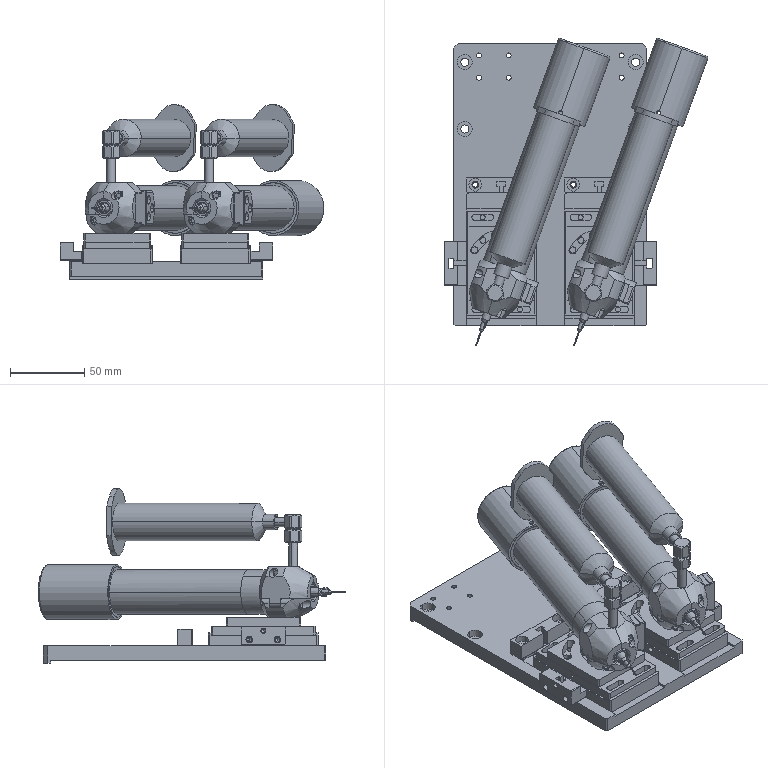Part | NX | features BREP 18 | 23 solids | 1038 faces | box 177.608 x 206.797 x 117.587 mm | volume 757600 mm3 | cylinder 498 | plane 428 | cone 86 | torus 16 | spline 10 | commonest cylinder face diameters 3.3 x72 4.5 x64 6 x36 2.5 x32 12 x32 1 x20